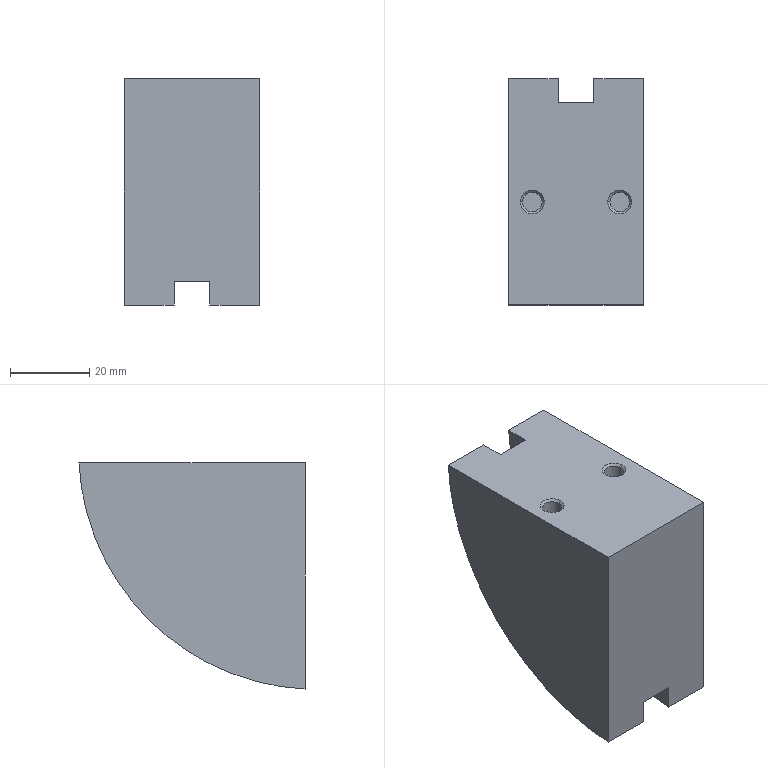Part | STEP file | Double-speed chain return rail VMH01-BS25-C206B Yihda 124-0 | 1 solid | 19 faces | box 34 x 56.925 x 56.925 mm | volume 78739 mm3 | plane 8 | cylinder 7 | cone 4 | commonest cylinder face diameters 4.917 x4 120 x2 108 x1
STEP:
#1=CARTESIAN_POINT('',(8.542,28.925,-28.));
#2=VERTEX_POINT('',#1);
#3=CARTESIAN_POINT('',(13.459,28.925,-28.));
#4=VERTEX_POINT('',#3);
#5=CARTESIAN_POINT('',(11.,28.925,-28.));
#6=DIRECTION('',(0.,0.,-1.));
#7=DIRECTION('',(-1.,0.,0.));
#8=AXIS2_PLACEMENT_3D('',#5,#6,#7);
#9=CIRCLE('',#8,2.459);
#10=EDGE_CURVE('',#2,#4,#9,.T.);
#11=ORIENTED_EDGE('',*,*,#10,.F.);
#12=CARTESIAN_POINT('',(11.,28.925,-28.));
#13=DIRECTION('',(0.,0.,-1.));
#14=DIRECTION('',(-1.,0.,0.));
#15=AXIS2_PLACEMENT_3D('',#12,#13,#14);
#16=CIRCLE('',#15,2.459);
#17=EDGE_CURVE('',#4,#2,#16,.T.);
#18=ORIENTED_EDGE('',*,*,#17,.F.);
#19=EDGE_LOOP('',(#11,#18));
#20=FACE_OUTER_BOUND('',#19,.T.);
#21=CARTESIAN_POINT('',(11.,31.383,-28.));
#22=DIRECTION('',(0.,0.,1.));
#23=DIRECTION('',(1.,0.,0.));
#24=AXIS2_PLACEMENT_3D('',#21,#22,#23);
#25=PLANE('',#24);
#26=ADVANCED_FACE('',(#20),#25,.T.);
#27=CARTESIAN_POINT('',(13.459,28.925,-3.542));
#28=VERTEX_POINT('',#27);
#29=CARTESIAN_POINT('',(8.542,28.925,-3.542));
#30=VERTEX_POINT('',#29);
#31=CARTESIAN_POINT('',(11.,28.925,-3.542));
#32=DIRECTION('',(0.,0.,-1.));
#33=DIRECTION('',(-1.,0.,0.));
#34=AXIS2_PLACEMENT_3D('',#31,#32,#33);
#35=CIRCLE('',#34,2.459);
#36=EDGE_CURVE('',#28,#30,#35,.T.);
#37=ORIENTED_EDGE('',*,*,#36,.F.);
#38=CARTESIAN_POINT('',(13.459,28.925,-28.));
#39=DIRECTION('',(0.,0.,1.));
#40=VECTOR('',#39,1000.);
#41=LINE('',#38,#40);
#42=EDGE_CURVE('',#4,#28,#41,.T.);
#43=ORIENTED_EDGE('',*,*,#42,.F.);
#44=ORIENTED_EDGE('',*,*,#17,.T.);
#45=CARTESIAN_POINT('',(8.542,28.925,-28.));
#46=DIRECTION('',(0.,0.,1.));
#47=VECTOR('',#46,1000.);
#48=LINE('',#45,#47);
#49=EDGE_CURVE('',#2,#30,#48,.T.);
#50=ORIENTED_EDGE('',*,*,#49,.T.);
#51=EDGE_LOOP('',(#37,#43,#44,#50));
#52=FACE_OUTER_BOUND('',#51,.T.);
#53=CARTESIAN_POINT('',(11.,28.925,-28.));
#54=DIRECTION('',(0.,0.,1.));
#55=DIRECTION('',(0.,1.,0.));
#56=AXIS2_PLACEMENT_3D('',#53,#54,#55);
#57=CYLINDRICAL_SURFACE('',#56,2.459);
#58=ADVANCED_FACE('',(#52),#57,.F.);
#59=ORIENTED_EDGE('',*,*,#10,.T.);
#60=ORIENTED_EDGE('',*,*,#42,.T.);
#61=CARTESIAN_POINT('',(11.,28.925,-3.542));
#62=DIRECTION('',(0.,0.,-1.));
#63=DIRECTION('',(-1.,0.,0.));
#64=AXIS2_PLACEMENT_3D('',#61,#62,#63);
#65=CIRCLE('',#64,2.459);
#66=EDGE_CURVE('',#30,#28,#65,.T.);
#67=ORIENTED_EDGE('',*,*,#66,.F.);
#68=ORIENTED_EDGE('',*,*,#49,.F.);
#69=EDGE_LOOP('',(#59,#60,#67,#68));
#70=FACE_OUTER_BOUND('',#69,.T.);
#71=CARTESIAN_POINT('',(11.,28.925,-28.));
#72=DIRECTION('',(0.,0.,1.));
#73=DIRECTION('',(0.,-1.,0.));
#74=AXIS2_PLACEMENT_3D('',#71,#72,#73);
#75=CYLINDRICAL_SURFACE('',#74,2.458);
#76=ADVANCED_FACE('',(#70),#75,.F.);
#77=ORIENTED_EDGE('',*,*,#66,.T.);
#78=CARTESIAN_POINT('',(14.,28.925,-3.));
#79=VERTEX_POINT('',#78);
#80=CARTESIAN_POINT('',(13.458,28.925,-3.541));
#81=DIRECTION('',(0.7071,0.,0.7071));
#82=VECTOR('',#81,1000.);
#83=LINE('',#80,#82);
#84=EDGE_CURVE('',#28,#79,#83,.T.);
#85=ORIENTED_EDGE('',*,*,#84,.T.);
#86=CARTESIAN_POINT('',(8.,28.925,-3.));
#87=VERTEX_POINT('',#86);
#88=CARTESIAN_POINT('',(11.,28.925,-3.));
#89=DIRECTION('',(0.,0.,-1.));
#90=DIRECTION('',(-1.,0.,0.));
#91=AXIS2_PLACEMENT_3D('',#88,#89,#90);
#92=CIRCLE('',#91,3.);
#93=EDGE_CURVE('',#87,#79,#92,.T.);
#94=ORIENTED_EDGE('',*,*,#93,.F.);
#95=CARTESIAN_POINT('',(8.542,28.925,-3.541));
#96=DIRECTION('',(-0.7071,0.,0.7071));
#97=VECTOR('',#96,1000.);
#98=LINE('',#95,#97);
#99=EDGE_CURVE('',#30,#87,#98,.T.);
#100=ORIENTED_EDGE('',*,*,#99,.F.);
#101=EDGE_LOOP('',(#77,#85,#94,#100));
#102=FACE_OUTER_BOUND('',#101,.T.);
#103=CARTESIAN_POINT('',(11.,28.925,-3.));
#104=DIRECTION('',(0.,0.,1.));
#105=DIRECTION('',(0.,-1.,0.));
#106=AXIS2_PLACEMENT_3D('',#103,#104,#105);
#107=CONICAL_SURFACE('',#106,3.,0.7854);
#108=ADVANCED_FACE('',(#102),#107,.F.);
#109=CARTESIAN_POINT('',(11.,28.925,-3.));
#110=DIRECTION('',(0.,0.,-1.));
#111=DIRECTION('',(-1.,0.,0.));
#112=AXIS2_PLACEMENT_3D('',#109,#110,#111);
#113=CIRCLE('',#112,3.);
#114=EDGE_CURVE('',#79,#87,#113,.T.);
#115=ORIENTED_EDGE('',*,*,#114,.F.);
#116=ORIENTED_EDGE('',*,*,#84,.F.);
#117=ORIENTED_EDGE('',*,*,#36,.T.);
#118=ORIENTED_EDGE('',*,*,#99,.T.);
#119=EDGE_LOOP('',(#115,#116,#117,#118));
#120=FACE_OUTER_BOUND('',#119,.T.);
#121=CARTESIAN_POINT('',(11.,28.925,-3.));
#122=DIRECTION('',(0.,0.,1.));
#123=DIRECTION('',(0.,1.,0.));
#124=AXIS2_PLACEMENT_3D('',#121,#122,#123);
#125=CONICAL_SURFACE('',#124,3.,0.7854);
#126=ADVANCED_FACE('',(#120),#125,.F.);
#127=ORIENTED_EDGE('',*,*,#93,.T.);
#128=ORIENTED_EDGE('',*,*,#114,.T.);
#129=EDGE_LOOP('',(#127,#128));
#130=FACE_BOUND('',#129,.T.);
#131=CARTESIAN_POINT('',(-14.,28.925,-3.));
#132=VERTEX_POINT('',#131);
#133=CARTESIAN_POINT('',(-8.,28.925,-3.));
#134=VERTEX_POINT('',#133);
#135=CARTESIAN_POINT('',(-11.,28.925,-3.));
#136=DIRECTION('',(0.,0.,-1.));
#137=DIRECTION('',(-1.,0.,0.));
#138=AXIS2_PLACEMENT_3D('',#135,#136,#137);
#139=CIRCLE('',#138,3.);
#140=EDGE_CURVE('',#132,#134,#139,.T.);
#141=ORIENTED_EDGE('',*,*,#140,.T.);
#142=CARTESIAN_POINT('',(-11.,28.925,-3.));
#143=DIRECTION('',(0.,0.,-1.));
#144=DIRECTION('',(-1.,0.,0.));
#145=AXIS2_PLACEMENT_3D('',#142,#143,#144);
#146=CIRCLE('',#145,3.);
#147=EDGE_CURVE('',#134,#132,#146,.T.);
#148=ORIENTED_EDGE('',*,*,#147,.T.);
#149=EDGE_LOOP('',(#141,#148));
#150=FACE_BOUND('',#149,.T.);
#151=CARTESIAN_POINT('',(17.,59.925,-3.));
#152=VERTEX_POINT('',#151);
#153=CARTESIAN_POINT('',(4.5,59.925,-3.));
#154=VERTEX_POINT('',#153);
#155=CARTESIAN_POINT('',(17.,59.925,-3.));
#156=DIRECTION('',(-1.,0.,0.));
#157=VECTOR('',#156,1000.);
#158=LINE('',#155,#157);
#159=EDGE_CURVE('',#152,#154,#158,.T.);
#160=ORIENTED_EDGE('',*,*,#159,.T.);
#161=CARTESIAN_POINT('',(4.5,53.917,-3.));
#162=VERTEX_POINT('',#161);
#163=CARTESIAN_POINT('',(4.5,59.925,-3.));
#164=DIRECTION('',(0.,-1.,0.));
#165=VECTOR('',#164,1000.);
#166=LINE('',#163,#165);
#167=EDGE_CURVE('',#154,#162,#166,.T.);
#168=ORIENTED_EDGE('',*,*,#167,.T.);
#169=CARTESIAN_POINT('',(-4.5,53.917,-3.));
#170=VERTEX_POINT('',#169);
#171=CARTESIAN_POINT('',(4.5,53.917,-3.));
#172=DIRECTION('',(-1.,0.,0.));
#173=VECTOR('',#172,1000.);
#174=LINE('',#171,#173);
#175=EDGE_CURVE('',#162,#170,#174,.T.);
#176=ORIENTED_EDGE('',*,*,#175,.T.);
#177=CARTESIAN_POINT('',(-4.5,59.925,-3.));
#178=VERTEX_POINT('',#177);
#179=CARTESIAN_POINT('',(-4.5,59.925,-3.));
#180=DIRECTION('',(0.,-1.,0.));
#181=VECTOR('',#180,1000.);
#182=LINE('',#179,#181);
#183=EDGE_CURVE('',#178,#170,#182,.T.);
#184=ORIENTED_EDGE('',*,*,#183,.F.);
#185=CARTESIAN_POINT('',(-17.,59.925,-3.));
#186=VERTEX_POINT('',#185);
#187=CARTESIAN_POINT('',(17.,59.925,-3.));
#188=DIRECTION('',(-1.,0.,0.));
#189=VECTOR('',#188,1000.);
#190=LINE('',#187,#189);
#191=EDGE_CURVE('',#178,#186,#190,.T.);
#192=ORIENTED_EDGE('',*,*,#191,.T.);
#193=CARTESIAN_POINT('',(-17.,3.,-3.));
#194=VERTEX_POINT('',#193);
#195=CARTESIAN_POINT('',(-17.,59.925,-3.));
#196=DIRECTION('',(0.,-1.,0.));
#197=VECTOR('',#196,1000.);
#198=LINE('',#195,#197);
#199=EDGE_CURVE('',#186,#194,#198,.T.);
#200=ORIENTED_EDGE('',*,*,#199,.T.);
#201=CARTESIAN_POINT('',(17.,3.,-3.));
#202=VERTEX_POINT('',#201);
#203=CARTESIAN_POINT('',(17.,3.,-3.));
#204=DIRECTION('',(-1.,0.,0.));
#205=VECTOR('',#204,1000.);
#206=LINE('',#203,#205);
#207=EDGE_CURVE('',#202,#194,#206,.T.);
#208=ORIENTED_EDGE('',*,*,#207,.F.);
#209=CARTESIAN_POINT('',(17.,59.925,-3.));
#210=DIRECTION('',(0.,-1.,0.));
#211=VECTOR('',#210,1000.);
#212=LINE('',#209,#211);
#213=EDGE_CURVE('',#152,#202,#212,.T.);
#214=ORIENTED_EDGE('',*,*,#213,.F.);
#215=EDGE_LOOP('',(#160,#168,#176,#184,#192,#200,#208,#214));
#216=FACE_OUTER_BOUND('',#215,.T.);
#217=CARTESIAN_POINT('',(17.,59.925,-3.));
#218=DIRECTION('',(0.,0.,-1.));
#219=DIRECTION('',(-1.,0.,0.));
#220=AXIS2_PLACEMENT_3D('',#217,#218,#219);
#221=PLANE('',#220);
#222=ADVANCED_FACE('',(#130,#150,#216),#221,.F.);
#223=ORIENTED_EDGE('',*,*,#213,.T.);
#224=CARTESIAN_POINT('',(17.,3.,-59.925));
#225=VERTEX_POINT('',#224);
#226=CARTESIAN_POINT('',(17.,3.,-3.));
#227=DIRECTION('',(0.,0.,-1.));
#228=VECTOR('',#227,1000.);
#229=LINE('',#226,#228);
#230=EDGE_CURVE('',#202,#225,#229,.T.);
#231=ORIENTED_EDGE('',*,*,#230,.T.);
#232=CARTESIAN_POINT('',(17.,0.,0.));
#233=DIRECTION('',(1.,0.,0.));
#234=DIRECTION('',(0.,0.,-1.));
#235=AXIS2_PLACEMENT_3D('',#232,#233,#234);
#236=CIRCLE('',#235,60.);
#237=EDGE_CURVE('',#225,#152,#236,.T.);
#238=ORIENTED_EDGE('',*,*,#237,.T.);
#239=EDGE_LOOP('',(#223,#231,#238));
#240=FACE_OUTER_BOUND('',#239,.T.);
#241=CARTESIAN_POINT('',(17.,0.,0.));
#242=DIRECTION('',(1.,0.,0.));
#243=DIRECTION('',(0.,0.,-1.));
#244=AXIS2_PLACEMENT_3D('',#241,#242,#243);
#245=PLANE('',#244);
#246=ADVANCED_FACE('',(#240),#245,.T.);
#247=CARTESIAN_POINT('',(4.5,3.,-59.925));
#248=VERTEX_POINT('',#247);
#249=CARTESIAN_POINT('',(17.,3.,-59.925));
#250=DIRECTION('',(-1.,0.,0.));
#251=VECTOR('',#250,1000.);
#252=LINE('',#249,#251);
#253=EDGE_CURVE('',#225,#248,#252,.T.);
#254=ORIENTED_EDGE('',*,*,#253,.T.);
#255=CARTESIAN_POINT('',(4.5,0.,0.));
#256=DIRECTION('',(1.,0.,0.));
#257=DIRECTION('',(0.,0.,-1.));
#258=AXIS2_PLACEMENT_3D('',#255,#256,#257);
#259=CIRCLE('',#258,60.);
#260=EDGE_CURVE('',#248,#154,#259,.T.);
#261=ORIENTED_EDGE('',*,*,#260,.T.);
#262=ORIENTED_EDGE('',*,*,#159,.F.);
#263=ORIENTED_EDGE('',*,*,#237,.F.);
#264=EDGE_LOOP('',(#254,#261,#262,#263));
#265=FACE_OUTER_BOUND('',#264,.T.);
#266=CARTESIAN_POINT('',(17.,0.,0.));
#267=DIRECTION('',(1.,0.,0.));
#268=DIRECTION('',(0.,-0.7071,0.7071));
#269=AXIS2_PLACEMENT_3D('',#266,#267,#268);
#270=CYLINDRICAL_SURFACE('',#269,60.);
#271=ADVANCED_FACE('',(#265),#270,.T.);
#272=ORIENTED_EDGE('',*,*,#260,.F.);
#273=CARTESIAN_POINT('',(4.5,3.,-53.917));
#274=VERTEX_POINT('',#273);
#275=CARTESIAN_POINT('',(4.5,3.,-53.917));
#276=DIRECTION('',(0.,0.,-1.));
#277=VECTOR('',#276,1000.);
#278=LINE('',#275,#277);
#279=EDGE_CURVE('',#274,#248,#278,.T.);
#280=ORIENTED_EDGE('',*,*,#279,.F.);
#281=CARTESIAN_POINT('',(4.5,0.,0.));
#282=DIRECTION('',(1.,0.,0.));
#283=DIRECTION('',(0.,0.,-1.));
#284=AXIS2_PLACEMENT_3D('',#281,#282,#283);
#285=CIRCLE('',#284,54.);
#286=EDGE_CURVE('',#274,#162,#285,.T.);
#287=ORIENTED_EDGE('',*,*,#286,.T.);
#288=ORIENTED_EDGE('',*,*,#167,.F.);
#289=EDGE_LOOP('',(#272,#280,#287,#288));
#290=FACE_OUTER_BOUND('',#289,.T.);
#291=CARTESIAN_POINT('',(4.5,0.,0.));
#292=DIRECTION('',(1.,0.,0.));
#293=DIRECTION('',(0.,0.,-1.));
#294=AXIS2_PLACEMENT_3D('',#291,#292,#293);
#295=PLANE('',#294);
#296=ADVANCED_FACE('',(#290),#295,.F.);
#297=CARTESIAN_POINT('',(-4.5,3.,-53.917));
#298=VERTEX_POINT('',#297);
#299=CARTESIAN_POINT('',(-4.5,0.,0.));
#300=DIRECTION('',(1.,0.,0.));
#301=DIRECTION('',(0.,0.,-1.));
#302=AXIS2_PLACEMENT_3D('',#299,#300,#301);
#303=CIRCLE('',#302,54.);
#304=EDGE_CURVE('',#298,#170,#303,.T.);
#305=ORIENTED_EDGE('',*,*,#304,.T.);
#306=ORIENTED_EDGE('',*,*,#175,.F.);
#307=ORIENTED_EDGE('',*,*,#286,.F.);
#308=CARTESIAN_POINT('',(4.5,3.,-53.917));
#309=DIRECTION('',(-1.,0.,0.));
#310=VECTOR('',#309,1000.);
#311=LINE('',#308,#310);
#312=EDGE_CURVE('',#274,#298,#311,.T.);
#313=ORIENTED_EDGE('',*,*,#312,.T.);
#314=EDGE_LOOP('',(#305,#306,#307,#313));
#315=FACE_OUTER_BOUND('',#314,.T.);
#316=CARTESIAN_POINT('',(4.5,0.,0.));
#317=DIRECTION('',(1.,0.,0.));
#318=DIRECTION('',(0.,-0.7071,0.7071));
#319=AXIS2_PLACEMENT_3D('',#316,#317,#318);
#320=CYLINDRICAL_SURFACE('',#319,54.);
#321=ADVANCED_FACE('',(#315),#320,.T.);
#322=ORIENTED_EDGE('',*,*,#312,.F.);
#323=ORIENTED_EDGE('',*,*,#279,.T.);
#324=ORIENTED_EDGE('',*,*,#253,.F.);
#325=ORIENTED_EDGE('',*,*,#230,.F.);
#326=ORIENTED_EDGE('',*,*,#207,.T.);
#327=CARTESIAN_POINT('',(-17.,3.,-59.925));
#328=VERTEX_POINT('',#327);
#329=CARTESIAN_POINT('',(-17.,3.,-3.));
#330=DIRECTION('',(0.,0.,-1.));
#331=VECTOR('',#330,1000.);
#332=LINE('',#329,#331);
#333=EDGE_CURVE('',#194,#328,#332,.T.);
#334=ORIENTED_EDGE('',*,*,#333,.T.);
#335=CARTESIAN_POINT('',(-4.5,3.,-59.925));
#336=VERTEX_POINT('',#335);
#337=CARTESIAN_POINT('',(17.,3.,-59.925));
#338=DIRECTION('',(-1.,0.,0.));
#339=VECTOR('',#338,1000.);
#340=LINE('',#337,#339);
#341=EDGE_CURVE('',#336,#328,#340,.T.);
#342=ORIENTED_EDGE('',*,*,#341,.F.);
#343=CARTESIAN_POINT('',(-4.5,3.,-53.917));
#344=DIRECTION('',(0.,0.,-1.));
#345=VECTOR('',#344,1000.);
#346=LINE('',#343,#345);
#347=EDGE_CURVE('',#298,#336,#346,.T.);
#348=ORIENTED_EDGE('',*,*,#347,.F.);
#349=EDGE_LOOP('',(#322,#323,#324,#325,#326,#334,#342,#348));
#350=FACE_OUTER_BOUND('',#349,.T.);
#351=CARTESIAN_POINT('',(17.,3.,-3.));
#352=DIRECTION('',(0.,1.,0.));
#353=DIRECTION('',(0.,0.,1.));
#354=AXIS2_PLACEMENT_3D('',#351,#352,#353);
#355=PLANE('',#354);
#356=ADVANCED_FACE('',(#350),#355,.F.);
#357=CARTESIAN_POINT('',(-4.5,0.,0.));
#358=DIRECTION('',(1.,0.,0.));
#359=DIRECTION('',(0.,0.,-1.));
#360=AXIS2_PLACEMENT_3D('',#357,#358,#359);
#361=CIRCLE('',#360,60.);
#362=EDGE_CURVE('',#336,#178,#361,.T.);
#363=ORIENTED_EDGE('',*,*,#362,.T.);
#364=ORIENTED_EDGE('',*,*,#183,.T.);
#365=ORIENTED_EDGE('',*,*,#304,.F.);
#366=ORIENTED_EDGE('',*,*,#347,.T.);
#367=EDGE_LOOP('',(#363,#364,#365,#366));
#368=FACE_OUTER_BOUND('',#367,.T.);
#369=CARTESIAN_POINT('',(-4.5,0.,0.));
#370=DIRECTION('',(1.,0.,0.));
#371=DIRECTION('',(0.,0.,-1.));
#372=AXIS2_PLACEMENT_3D('',#369,#370,#371);
#373=PLANE('',#372);
#374=ADVANCED_FACE('',(#368),#373,.T.);
#375=ORIENTED_EDGE('',*,*,#362,.F.);
#376=ORIENTED_EDGE('',*,*,#341,.T.);
#377=CARTESIAN_POINT('',(-17.,0.,0.));
#378=DIRECTION('',(1.,0.,0.));
#379=DIRECTION('',(0.,0.,-1.));
#380=AXIS2_PLACEMENT_3D('',#377,#378,#379);
#381=CIRCLE('',#380,60.);
#382=EDGE_CURVE('',#328,#186,#381,.T.);
#383=ORIENTED_EDGE('',*,*,#382,.T.);
#384=ORIENTED_EDGE('',*,*,#191,.F.);
#385=EDGE_LOOP('',(#375,#376,#383,#384));
#386=FACE_OUTER_BOUND('',#385,.T.);
#387=CARTESIAN_POINT('',(17.,0.,0.));
#388=DIRECTION('',(1.,0.,0.));
#389=DIRECTION('',(0.,-0.7071,0.7071));
#390=AXIS2_PLACEMENT_3D('',#387,#388,#389);
#391=CYLINDRICAL_SURFACE('',#390,60.);
#392=ADVANCED_FACE('',(#386),#391,.T.);
#393=ORIENTED_EDGE('',*,*,#199,.F.);
#394=ORIENTED_EDGE('',*,*,#382,.F.);
#395=ORIENTED_EDGE('',*,*,#333,.F.);
#396=EDGE_LOOP('',(#393,#394,#395));
#397=FACE_OUTER_BOUND('',#396,.T.);
#398=CARTESIAN_POINT('',(-17.,0.,0.));
#399=DIRECTION('',(1.,0.,0.));
#400=DIRECTION('',(0.,0.,-1.));
#401=AXIS2_PLACEMENT_3D('',#398,#399,#400);
#402=PLANE('',#401);
#403=ADVANCED_FACE('',(#397),#402,.F.);
#404=ORIENTED_EDGE('',*,*,#147,.F.);
#405=CARTESIAN_POINT('',(-8.542,28.925,-3.541));
#406=VERTEX_POINT('',#405);
#407=CARTESIAN_POINT('',(-8.542,28.925,-3.541));
#408=DIRECTION('',(0.7071,0.,0.7071));
#409=VECTOR('',#408,1000.);
#410=LINE('',#407,#409);
#411=EDGE_CURVE('',#406,#134,#410,.T.);
#412=ORIENTED_EDGE('',*,*,#411,.F.);
#413=CARTESIAN_POINT('',(-13.459,28.925,-3.542));
#414=VERTEX_POINT('',#413);
#415=CARTESIAN_POINT('',(-11.,28.925,-3.542));
#416=DIRECTION('',(0.,0.,-1.));
#417=DIRECTION('',(-1.,0.,0.));
#418=AXIS2_PLACEMENT_3D('',#415,#416,#417);
#419=CIRCLE('',#418,2.459);
#420=EDGE_CURVE('',#406,#414,#419,.T.);
#421=ORIENTED_EDGE('',*,*,#420,.T.);
#422=CARTESIAN_POINT('',(-13.458,28.925,-3.541));
#423=DIRECTION('',(-0.7071,0.,0.7071));
#424=VECTOR('',#423,1000.);
#425=LINE('',#422,#424);
#426=EDGE_CURVE('',#414,#132,#425,.T.);
#427=ORIENTED_EDGE('',*,*,#426,.T.);
#428=EDGE_LOOP('',(#404,#412,#421,#427));
#429=FACE_OUTER_BOUND('',#428,.T.);
#430=CARTESIAN_POINT('',(-11.,28.925,-3.));
#431=DIRECTION('',(0.,0.,1.));
#432=DIRECTION('',(0.,1.,0.));
#433=AXIS2_PLACEMENT_3D('',#430,#431,#432);
#434=CONICAL_SURFACE('',#433,3.,0.7854);
#435=ADVANCED_FACE('',(#429),#434,.F.);
#436=CARTESIAN_POINT('',(-11.,28.925,-3.542));
#437=DIRECTION('',(0.,0.,-1.));
#438=DIRECTION('',(-1.,0.,0.));
#439=AXIS2_PLACEMENT_3D('',#436,#437,#438);
#440=CIRCLE('',#439,2.459);
#441=EDGE_CURVE('',#414,#406,#440,.T.);
#442=ORIENTED_EDGE('',*,*,#441,.T.);
#443=ORIENTED_EDGE('',*,*,#411,.T.);
#444=ORIENTED_EDGE('',*,*,#140,.F.);
#445=ORIENTED_EDGE('',*,*,#426,.F.);
#446=EDGE_LOOP('',(#442,#443,#444,#445));
#447=FACE_OUTER_BOUND('',#446,.T.);
#448=CARTESIAN_POINT('',(-11.,28.925,-3.));
#449=DIRECTION('',(0.,0.,1.));
#450=DIRECTION('',(0.,-1.,0.));
#451=AXIS2_PLACEMENT_3D('',#448,#449,#450);
#452=CONICAL_SURFACE('',#451,3.,0.7854);
#453=ADVANCED_FACE('',(#447),#452,.F.);
#454=CARTESIAN_POINT('',(-13.459,28.925,-28.));
#455=VERTEX_POINT('',#454);
#456=CARTESIAN_POINT('',(-8.542,28.925,-28.));
#457=VERTEX_POINT('',#456);
#458=CARTESIAN_POINT('',(-11.,28.925,-28.));
#459=DIRECTION('',(0.,0.,-1.));
#460=DIRECTION('',(-1.,0.,0.));
#461=AXIS2_PLACEMENT_3D('',#458,#459,#460);
#462=CIRCLE('',#461,2.459);
#463=EDGE_CURVE('',#455,#457,#462,.T.);
#464=ORIENTED_EDGE('',*,*,#463,.T.);
#465=CARTESIAN_POINT('',(-8.542,28.925,-28.));
#466=DIRECTION('',(0.,0.,1.));
#467=VECTOR('',#466,1000.);
#468=LINE('',#465,#467);
#469=EDGE_CURVE('',#457,#406,#468,.T.);
#470=ORIENTED_EDGE('',*,*,#469,.T.);
#471=ORIENTED_EDGE('',*,*,#441,.F.);
#472=CARTESIAN_POINT('',(-13.459,28.925,-28.));
#473=DIRECTION('',(0.,0.,1.));
#474=VECTOR('',#473,1000.);
#475=LINE('',#472,#474);
#476=EDGE_CURVE('',#455,#414,#475,.T.);
#477=ORIENTED_EDGE('',*,*,#476,.F.);
#478=EDGE_LOOP('',(#464,#470,#471,#477));
#479=FACE_OUTER_BOUND('',#478,.T.);
#480=CARTESIAN_POINT('',(-11.,28.925,-28.));
#481=DIRECTION('',(0.,0.,1.));
#482=DIRECTION('',(0.,-1.,0.));
#483=AXIS2_PLACEMENT_3D('',#480,#481,#482);
#484=CYLINDRICAL_SURFACE('',#483,2.458);
#485=ADVANCED_FACE('',(#479),#484,.F.);
#486=ORIENTED_EDGE('',*,*,#420,.F.);
#487=ORIENTED_EDGE('',*,*,#469,.F.);
#488=CARTESIAN_POINT('',(-11.,28.925,-28.));
#489=DIRECTION('',(0.,0.,-1.));
#490=DIRECTION('',(-1.,0.,0.));
#491=AXIS2_PLACEMENT_3D('',#488,#489,#490);
#492=CIRCLE('',#491,2.459);
#493=EDGE_CURVE('',#457,#455,#492,.T.);
#494=ORIENTED_EDGE('',*,*,#493,.T.);
#495=ORIENTED_EDGE('',*,*,#476,.T.);
#496=EDGE_LOOP('',(#486,#487,#494,#495));
#497=FACE_OUTER_BOUND('',#496,.T.);
#498=CARTESIAN_POINT('',(-11.,28.925,-28.));
#499=DIRECTION('',(0.,0.,1.));
#500=DIRECTION('',(0.,1.,0.));
#501=AXIS2_PLACEMENT_3D('',#498,#499,#500);
#502=CYLINDRICAL_SURFACE('',#501,2.459);
#503=ADVANCED_FACE('',(#497),#502,.F.);
#504=ORIENTED_EDGE('',*,*,#463,.F.);
#505=ORIENTED_EDGE('',*,*,#493,.F.);
#506=EDGE_LOOP('',(#504,#505));
#507=FACE_OUTER_BOUND('',#506,.T.);
#508=CARTESIAN_POINT('',(-11.,31.383,-28.));
#509=DIRECTION('',(0.,0.,1.));
#510=DIRECTION('',(1.,0.,0.));
#511=AXIS2_PLACEMENT_3D('',#508,#509,#510);
#512=PLANE('',#511);
#513=ADVANCED_FACE('',(#507),#512,.T.);
#514=CLOSED_SHELL('',(#26,#58,#76,#108,#126,#222,#246,#271,#296,#321,#356,#374,#392,#403,#435,#453,#485,#503,#513));
#515=MANIFOLD_SOLID_BREP('',#514);
#516=CARTESIAN_POINT('',(0.,0.,0.));
#517=DIRECTION('',(0.,0.,1.));
#518=DIRECTION('',(1.,0.,0.));
#519=AXIS2_PLACEMENT_3D('',#516,#517,#518);
#520=(LENGTH_UNIT()NAMED_UNIT(*)SI_UNIT(.MILLI.,.METRE.));
#521=UNCERTAINTY_MEASURE_WITH_UNIT(LENGTH_MEASURE(0.00001),#520,'','');
#522=(NAMED_UNIT(*)PLANE_ANGLE_UNIT()SI_UNIT($,.RADIAN.));
#523=(NAMED_UNIT(*)SI_UNIT($,.STERADIAN.)SOLID_ANGLE_UNIT());
#524=(GEOMETRIC_REPRESENTATION_CONTEXT(3)GLOBAL_UNCERTAINTY_ASSIGNED_CONTEXT((#521))GLOBAL_UNIT_ASSIGNED_CONTEXT((#520,#522,#523))REPRESENTATION_CONTEXT('',''));
#525=ADVANCED_BREP_SHAPE_REPRESENTATION('',(#515,#519),#524);